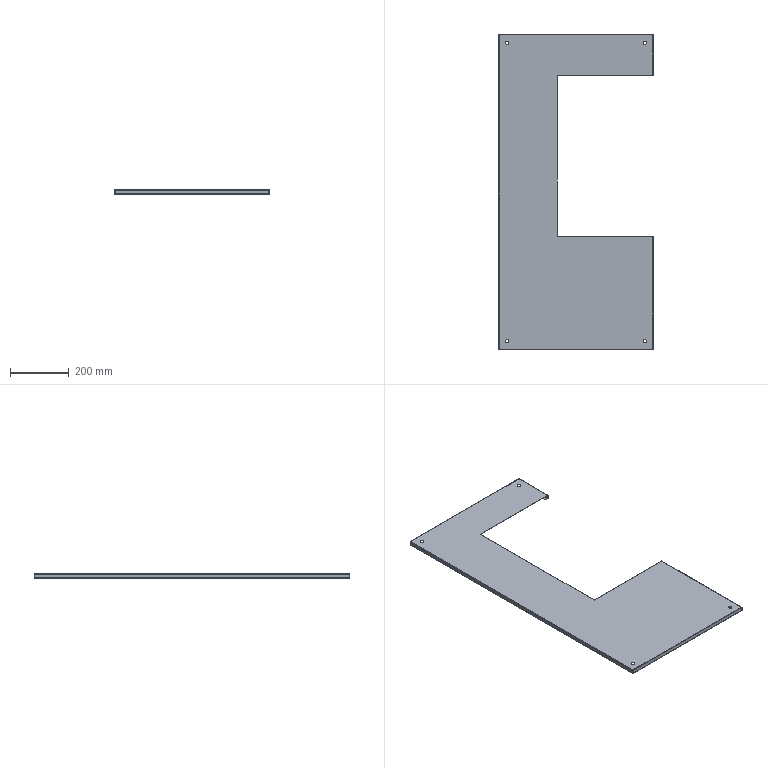Part | STEP file | lower frame left cover plate | 1 solid | 106 faces | box 527 x 1077 x 15 mm | volume 446588 mm3 | plane 66 | cylinder 28 | spline 12 | commonest cylinder face diameters 0.2 x10 2.2 x10 11.5 x8